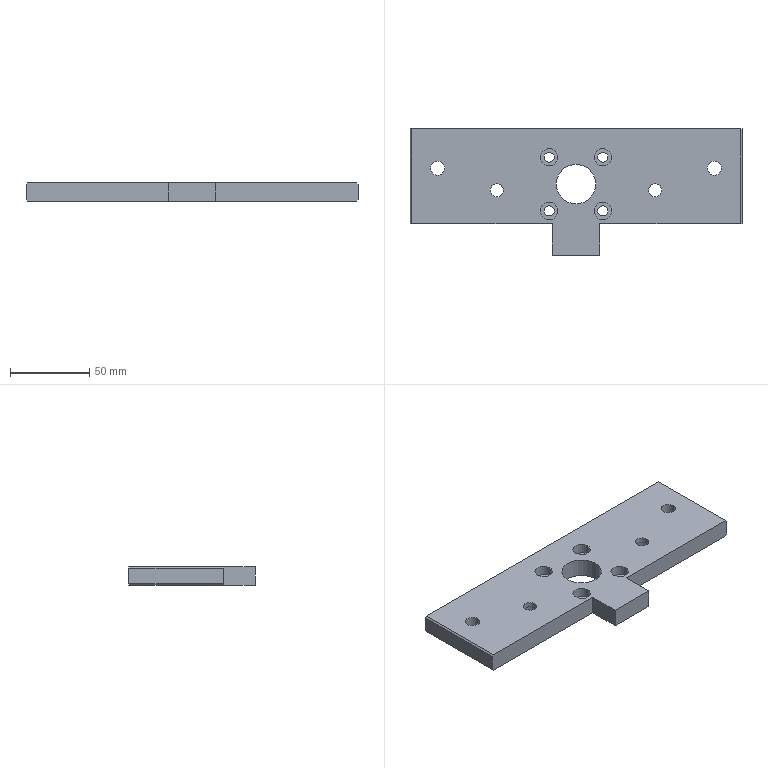Part | SolidWorks | features HoleWzd 3, Chamfer 1, Cut 1, Extrusion 1, ICE 1 | 1 solid | 50 faces | box 210 x 80 x 12 mm | volume 144293 mm3 | cylinder 30 | plane 20 | commonest cylinder face diameters 6.4 x8 11 x8 8.4 x4 9 x4 15 x4 25 x2
STEP:
#1=CARTESIAN_POINT('',(197.,35.,12.));
#2=VERTEX_POINT('',#1);
#3=CARTESIAN_POINT('',(188.,35.,12.));
#4=VERTEX_POINT('',#3);
#5=CARTESIAN_POINT('',(192.5,35.,12.));
#6=DIRECTION('',(0.,0.,-1.));
#7=DIRECTION('',(-1.,0.,0.));
#8=AXIS2_PLACEMENT_3D('',#5,#6,#7);
#9=CIRCLE('',#8,4.5);
#10=EDGE_CURVE('',#2,#4,#9,.T.);
#11=ORIENTED_EDGE('',*,*,#10,.F.);
#12=CARTESIAN_POINT('',(197.,35.,0.));
#13=VERTEX_POINT('',#12);
#14=CARTESIAN_POINT('',(197.,35.,0.));
#15=DIRECTION('',(0.,0.,-1.));
#16=VECTOR('',#15,1000.);
#17=LINE('',#14,#16);
#18=EDGE_CURVE('',#2,#13,#17,.T.);
#19=ORIENTED_EDGE('',*,*,#18,.T.);
#20=CARTESIAN_POINT('',(188.,35.,0.));
#21=VERTEX_POINT('',#20);
#22=CARTESIAN_POINT('',(192.5,35.,0.));
#23=DIRECTION('',(0.,0.,-1.));
#24=DIRECTION('',(-1.,0.,0.));
#25=AXIS2_PLACEMENT_3D('',#22,#23,#24);
#26=CIRCLE('',#25,4.5);
#27=EDGE_CURVE('',#13,#21,#26,.T.);
#28=ORIENTED_EDGE('',*,*,#27,.T.);
#29=CARTESIAN_POINT('',(188.,35.,0.));
#30=DIRECTION('',(0.,0.,-1.));
#31=VECTOR('',#30,1000.);
#32=LINE('',#29,#31);
#33=EDGE_CURVE('',#4,#21,#32,.T.);
#34=ORIENTED_EDGE('',*,*,#33,.F.);
#35=EDGE_LOOP('',(#11,#19,#28,#34));
#36=FACE_OUTER_BOUND('',#35,.T.);
#37=CARTESIAN_POINT('',(192.5,35.,0.));
#38=DIRECTION('',(0.,0.,-1.));
#39=DIRECTION('',(-1.,0.,0.));
#40=AXIS2_PLACEMENT_3D('',#37,#38,#39);
#41=CYLINDRICAL_SURFACE('',#40,4.5);
#42=ADVANCED_FACE('',(#36),#41,.F.);
#43=CARTESIAN_POINT('',(22.,35.,12.));
#44=VERTEX_POINT('',#43);
#45=CARTESIAN_POINT('',(13.,35.,12.));
#46=VERTEX_POINT('',#45);
#47=CARTESIAN_POINT('',(17.5,35.,12.));
#48=DIRECTION('',(0.,0.,-1.));
#49=DIRECTION('',(-1.,0.,0.));
#50=AXIS2_PLACEMENT_3D('',#47,#48,#49);
#51=CIRCLE('',#50,4.5);
#52=EDGE_CURVE('',#44,#46,#51,.T.);
#53=ORIENTED_EDGE('',*,*,#52,.F.);
#54=CARTESIAN_POINT('',(22.,35.,0.));
#55=VERTEX_POINT('',#54);
#56=CARTESIAN_POINT('',(22.,35.,0.));
#57=DIRECTION('',(0.,0.,-1.));
#58=VECTOR('',#57,1000.);
#59=LINE('',#56,#58);
#60=EDGE_CURVE('',#44,#55,#59,.T.);
#61=ORIENTED_EDGE('',*,*,#60,.T.);
#62=CARTESIAN_POINT('',(13.,35.,0.));
#63=VERTEX_POINT('',#62);
#64=CARTESIAN_POINT('',(17.5,35.,0.));
#65=DIRECTION('',(0.,0.,-1.));
#66=DIRECTION('',(-1.,0.,0.));
#67=AXIS2_PLACEMENT_3D('',#64,#65,#66);
#68=CIRCLE('',#67,4.5);
#69=EDGE_CURVE('',#55,#63,#68,.T.);
#70=ORIENTED_EDGE('',*,*,#69,.T.);
#71=CARTESIAN_POINT('',(13.,35.,0.));
#72=DIRECTION('',(0.,0.,-1.));
#73=VECTOR('',#72,1000.);
#74=LINE('',#71,#73);
#75=EDGE_CURVE('',#46,#63,#74,.T.);
#76=ORIENTED_EDGE('',*,*,#75,.F.);
#77=EDGE_LOOP('',(#53,#61,#70,#76));
#78=FACE_OUTER_BOUND('',#77,.T.);
#79=CARTESIAN_POINT('',(17.5,35.,0.));
#80=DIRECTION('',(0.,0.,-1.));
#81=DIRECTION('',(-1.,0.,0.));
#82=AXIS2_PLACEMENT_3D('',#79,#80,#81);
#83=CYLINDRICAL_SURFACE('',#82,4.5);
#84=ADVANCED_FACE('',(#78),#83,.F.);
#85=CARTESIAN_POINT('',(116.5,42.,5.6));
#86=VERTEX_POINT('',#85);
#87=CARTESIAN_POINT('',(127.5,42.,5.6));
#88=VERTEX_POINT('',#87);
#89=CARTESIAN_POINT('',(122.,42.,5.6));
#90=DIRECTION('',(0.,0.,1.));
#91=DIRECTION('',(1.,0.,0.));
#92=AXIS2_PLACEMENT_3D('',#89,#90,#91);
#93=CIRCLE('',#92,5.5);
#94=EDGE_CURVE('',#86,#88,#93,.T.);
#95=ORIENTED_EDGE('',*,*,#94,.F.);
#96=CARTESIAN_POINT('',(116.5,42.,12.));
#97=VERTEX_POINT('',#96);
#98=CARTESIAN_POINT('',(116.5,42.,12.));
#99=DIRECTION('',(0.,0.,1.));
#100=VECTOR('',#99,1000.);
#101=LINE('',#98,#100);
#102=EDGE_CURVE('',#86,#97,#101,.T.);
#103=ORIENTED_EDGE('',*,*,#102,.T.);
#104=CARTESIAN_POINT('',(127.5,42.,12.));
#105=VERTEX_POINT('',#104);
#106=CARTESIAN_POINT('',(122.,42.,12.));
#107=DIRECTION('',(0.,0.,1.));
#108=DIRECTION('',(1.,0.,0.));
#109=AXIS2_PLACEMENT_3D('',#106,#107,#108);
#110=CIRCLE('',#109,5.5);
#111=EDGE_CURVE('',#97,#105,#110,.T.);
#112=ORIENTED_EDGE('',*,*,#111,.T.);
#113=CARTESIAN_POINT('',(127.5,42.,12.));
#114=DIRECTION('',(0.,0.,1.));
#115=VECTOR('',#114,1000.);
#116=LINE('',#113,#115);
#117=EDGE_CURVE('',#88,#105,#116,.T.);
#118=ORIENTED_EDGE('',*,*,#117,.F.);
#119=EDGE_LOOP('',(#95,#103,#112,#118));
#120=FACE_OUTER_BOUND('',#119,.T.);
#121=CARTESIAN_POINT('',(122.,42.,12.));
#122=DIRECTION('',(0.,0.,1.));
#123=DIRECTION('',(1.,0.,0.));
#124=AXIS2_PLACEMENT_3D('',#121,#122,#123);
#125=CYLINDRICAL_SURFACE('',#124,5.5);
#126=ADVANCED_FACE('',(#120),#125,.F.);
#127=CARTESIAN_POINT('',(118.8,42.,0.));
#128=VERTEX_POINT('',#127);
#129=CARTESIAN_POINT('',(125.2,42.,0.));
#130=VERTEX_POINT('',#129);
#131=CARTESIAN_POINT('',(122.,42.,0.));
#132=DIRECTION('',(0.,0.,1.));
#133=DIRECTION('',(1.,0.,0.));
#134=AXIS2_PLACEMENT_3D('',#131,#132,#133);
#135=CIRCLE('',#134,3.2);
#136=EDGE_CURVE('',#128,#130,#135,.T.);
#137=ORIENTED_EDGE('',*,*,#136,.F.);
#138=CARTESIAN_POINT('',(118.8,42.,5.6));
#139=VERTEX_POINT('',#138);
#140=CARTESIAN_POINT('',(118.8,42.,12.));
#141=DIRECTION('',(0.,0.,1.));
#142=VECTOR('',#141,1000.);
#143=LINE('',#140,#142);
#144=EDGE_CURVE('',#128,#139,#143,.T.);
#145=ORIENTED_EDGE('',*,*,#144,.T.);
#146=CARTESIAN_POINT('',(125.2,42.,5.6));
#147=VERTEX_POINT('',#146);
#148=CARTESIAN_POINT('',(122.,42.,5.6));
#149=DIRECTION('',(0.,0.,1.));
#150=DIRECTION('',(1.,0.,0.));
#151=AXIS2_PLACEMENT_3D('',#148,#149,#150);
#152=CIRCLE('',#151,3.2);
#153=EDGE_CURVE('',#139,#147,#152,.T.);
#154=ORIENTED_EDGE('',*,*,#153,.T.);
#155=CARTESIAN_POINT('',(125.2,42.,12.));
#156=DIRECTION('',(0.,0.,1.));
#157=VECTOR('',#156,1000.);
#158=LINE('',#155,#157);
#159=EDGE_CURVE('',#130,#147,#158,.T.);
#160=ORIENTED_EDGE('',*,*,#159,.F.);
#161=EDGE_LOOP('',(#137,#145,#154,#160));
#162=FACE_OUTER_BOUND('',#161,.T.);
#163=CARTESIAN_POINT('',(122.,42.,12.));
#164=DIRECTION('',(0.,0.,1.));
#165=DIRECTION('',(1.,0.,0.));
#166=AXIS2_PLACEMENT_3D('',#163,#164,#165);
#167=CYLINDRICAL_SURFACE('',#166,3.2);
#168=ADVANCED_FACE('',(#162),#167,.F.);
#169=CARTESIAN_POINT('',(82.5,42.,5.6));
#170=VERTEX_POINT('',#169);
#171=CARTESIAN_POINT('',(93.5,42.,5.6));
#172=VERTEX_POINT('',#171);
#173=CARTESIAN_POINT('',(88.,42.,5.6));
#174=DIRECTION('',(0.,0.,1.));
#175=DIRECTION('',(1.,0.,0.));
#176=AXIS2_PLACEMENT_3D('',#173,#174,#175);
#177=CIRCLE('',#176,5.5);
#178=EDGE_CURVE('',#170,#172,#177,.T.);
#179=ORIENTED_EDGE('',*,*,#178,.F.);
#180=CARTESIAN_POINT('',(82.5,42.,12.));
#181=VERTEX_POINT('',#180);
#182=CARTESIAN_POINT('',(82.5,42.,12.));
#183=DIRECTION('',(0.,0.,1.));
#184=VECTOR('',#183,1000.);
#185=LINE('',#182,#184);
#186=EDGE_CURVE('',#170,#181,#185,.T.);
#187=ORIENTED_EDGE('',*,*,#186,.T.);
#188=CARTESIAN_POINT('',(93.5,42.,12.));
#189=VERTEX_POINT('',#188);
#190=CARTESIAN_POINT('',(88.,42.,12.));
#191=DIRECTION('',(0.,0.,1.));
#192=DIRECTION('',(1.,0.,0.));
#193=AXIS2_PLACEMENT_3D('',#190,#191,#192);
#194=CIRCLE('',#193,5.5);
#195=EDGE_CURVE('',#181,#189,#194,.T.);
#196=ORIENTED_EDGE('',*,*,#195,.T.);
#197=CARTESIAN_POINT('',(93.5,42.,12.));
#198=DIRECTION('',(0.,0.,1.));
#199=VECTOR('',#198,1000.);
#200=LINE('',#197,#199);
#201=EDGE_CURVE('',#172,#189,#200,.T.);
#202=ORIENTED_EDGE('',*,*,#201,.F.);
#203=EDGE_LOOP('',(#179,#187,#196,#202));
#204=FACE_OUTER_BOUND('',#203,.T.);
#205=CARTESIAN_POINT('',(88.,42.,12.));
#206=DIRECTION('',(0.,0.,1.));
#207=DIRECTION('',(1.,0.,0.));
#208=AXIS2_PLACEMENT_3D('',#205,#206,#207);
#209=CYLINDRICAL_SURFACE('',#208,5.5);
#210=ADVANCED_FACE('',(#204),#209,.F.);
#211=CARTESIAN_POINT('',(84.8,42.,0.));
#212=VERTEX_POINT('',#211);
#213=CARTESIAN_POINT('',(91.2,42.,0.));
#214=VERTEX_POINT('',#213);
#215=CARTESIAN_POINT('',(88.,42.,0.));
#216=DIRECTION('',(0.,0.,1.));
#217=DIRECTION('',(1.,0.,0.));
#218=AXIS2_PLACEMENT_3D('',#215,#216,#217);
#219=CIRCLE('',#218,3.2);
#220=EDGE_CURVE('',#212,#214,#219,.T.);
#221=ORIENTED_EDGE('',*,*,#220,.F.);
#222=CARTESIAN_POINT('',(84.8,42.,5.6));
#223=VERTEX_POINT('',#222);
#224=CARTESIAN_POINT('',(84.8,42.,12.));
#225=DIRECTION('',(0.,0.,1.));
#226=VECTOR('',#225,1000.);
#227=LINE('',#224,#226);
#228=EDGE_CURVE('',#212,#223,#227,.T.);
#229=ORIENTED_EDGE('',*,*,#228,.T.);
#230=CARTESIAN_POINT('',(91.2,42.,5.6));
#231=VERTEX_POINT('',#230);
#232=CARTESIAN_POINT('',(88.,42.,5.6));
#233=DIRECTION('',(0.,0.,1.));
#234=DIRECTION('',(1.,0.,0.));
#235=AXIS2_PLACEMENT_3D('',#232,#233,#234);
#236=CIRCLE('',#235,3.2);
#237=EDGE_CURVE('',#223,#231,#236,.T.);
#238=ORIENTED_EDGE('',*,*,#237,.T.);
#239=CARTESIAN_POINT('',(91.2,42.,12.));
#240=DIRECTION('',(0.,0.,1.));
#241=VECTOR('',#240,1000.);
#242=LINE('',#239,#241);
#243=EDGE_CURVE('',#214,#231,#242,.T.);
#244=ORIENTED_EDGE('',*,*,#243,.F.);
#245=EDGE_LOOP('',(#221,#229,#238,#244));
#246=FACE_OUTER_BOUND('',#245,.T.);
#247=CARTESIAN_POINT('',(88.,42.,12.));
#248=DIRECTION('',(0.,0.,1.));
#249=DIRECTION('',(1.,0.,0.));
#250=AXIS2_PLACEMENT_3D('',#247,#248,#249);
#251=CYLINDRICAL_SURFACE('',#250,3.2);
#252=ADVANCED_FACE('',(#246),#251,.F.);
#253=CARTESIAN_POINT('',(116.5,8.,5.6));
#254=VERTEX_POINT('',#253);
#255=CARTESIAN_POINT('',(127.5,8.,5.6));
#256=VERTEX_POINT('',#255);
#257=CARTESIAN_POINT('',(122.,8.,5.6));
#258=DIRECTION('',(0.,0.,1.));
#259=DIRECTION('',(1.,0.,0.));
#260=AXIS2_PLACEMENT_3D('',#257,#258,#259);
#261=CIRCLE('',#260,5.5);
#262=EDGE_CURVE('',#254,#256,#261,.T.);
#263=ORIENTED_EDGE('',*,*,#262,.F.);
#264=CARTESIAN_POINT('',(116.5,8.,12.));
#265=VERTEX_POINT('',#264);
#266=CARTESIAN_POINT('',(116.5,8.,12.));
#267=DIRECTION('',(0.,0.,1.));
#268=VECTOR('',#267,1000.);
#269=LINE('',#266,#268);
#270=EDGE_CURVE('',#254,#265,#269,.T.);
#271=ORIENTED_EDGE('',*,*,#270,.T.);
#272=CARTESIAN_POINT('',(127.5,8.,12.));
#273=VERTEX_POINT('',#272);
#274=CARTESIAN_POINT('',(122.,8.,12.));
#275=DIRECTION('',(0.,0.,1.));
#276=DIRECTION('',(1.,0.,0.));
#277=AXIS2_PLACEMENT_3D('',#274,#275,#276);
#278=CIRCLE('',#277,5.5);
#279=EDGE_CURVE('',#265,#273,#278,.T.);
#280=ORIENTED_EDGE('',*,*,#279,.T.);
#281=CARTESIAN_POINT('',(127.5,8.,12.));
#282=DIRECTION('',(0.,0.,1.));
#283=VECTOR('',#282,1000.);
#284=LINE('',#281,#283);
#285=EDGE_CURVE('',#256,#273,#284,.T.);
#286=ORIENTED_EDGE('',*,*,#285,.F.);
#287=EDGE_LOOP('',(#263,#271,#280,#286));
#288=FACE_OUTER_BOUND('',#287,.T.);
#289=CARTESIAN_POINT('',(122.,8.,12.));
#290=DIRECTION('',(0.,0.,1.));
#291=DIRECTION('',(1.,0.,0.));
#292=AXIS2_PLACEMENT_3D('',#289,#290,#291);
#293=CYLINDRICAL_SURFACE('',#292,5.5);
#294=ADVANCED_FACE('',(#288),#293,.F.);
#295=CARTESIAN_POINT('',(118.8,8.,0.));
#296=VERTEX_POINT('',#295);
#297=CARTESIAN_POINT('',(125.2,8.,0.));
#298=VERTEX_POINT('',#297);
#299=CARTESIAN_POINT('',(122.,8.,0.));
#300=DIRECTION('',(0.,0.,1.));
#301=DIRECTION('',(1.,0.,0.));
#302=AXIS2_PLACEMENT_3D('',#299,#300,#301);
#303=CIRCLE('',#302,3.2);
#304=EDGE_CURVE('',#296,#298,#303,.T.);
#305=ORIENTED_EDGE('',*,*,#304,.F.);
#306=CARTESIAN_POINT('',(118.8,8.,5.6));
#307=VERTEX_POINT('',#306);
#308=CARTESIAN_POINT('',(118.8,8.,12.));
#309=DIRECTION('',(0.,0.,1.));
#310=VECTOR('',#309,1000.);
#311=LINE('',#308,#310);
#312=EDGE_CURVE('',#296,#307,#311,.T.);
#313=ORIENTED_EDGE('',*,*,#312,.T.);
#314=CARTESIAN_POINT('',(125.2,8.,5.6));
#315=VERTEX_POINT('',#314);
#316=CARTESIAN_POINT('',(122.,8.,5.6));
#317=DIRECTION('',(0.,0.,1.));
#318=DIRECTION('',(1.,0.,0.));
#319=AXIS2_PLACEMENT_3D('',#316,#317,#318);
#320=CIRCLE('',#319,3.2);
#321=EDGE_CURVE('',#307,#315,#320,.T.);
#322=ORIENTED_EDGE('',*,*,#321,.T.);
#323=CARTESIAN_POINT('',(125.2,8.,12.));
#324=DIRECTION('',(0.,0.,1.));
#325=VECTOR('',#324,1000.);
#326=LINE('',#323,#325);
#327=EDGE_CURVE('',#298,#315,#326,.T.);
#328=ORIENTED_EDGE('',*,*,#327,.F.);
#329=EDGE_LOOP('',(#305,#313,#322,#328));
#330=FACE_OUTER_BOUND('',#329,.T.);
#331=CARTESIAN_POINT('',(122.,8.,12.));
#332=DIRECTION('',(0.,0.,1.));
#333=DIRECTION('',(1.,0.,0.));
#334=AXIS2_PLACEMENT_3D('',#331,#332,#333);
#335=CYLINDRICAL_SURFACE('',#334,3.2);
#336=ADVANCED_FACE('',(#330),#335,.F.);
#337=CARTESIAN_POINT('',(82.5,8.,5.6));
#338=VERTEX_POINT('',#337);
#339=CARTESIAN_POINT('',(93.5,8.,5.6));
#340=VERTEX_POINT('',#339);
#341=CARTESIAN_POINT('',(88.,8.,5.6));
#342=DIRECTION('',(0.,0.,1.));
#343=DIRECTION('',(1.,0.,0.));
#344=AXIS2_PLACEMENT_3D('',#341,#342,#343);
#345=CIRCLE('',#344,5.5);
#346=EDGE_CURVE('',#338,#340,#345,.T.);
#347=ORIENTED_EDGE('',*,*,#346,.F.);
#348=CARTESIAN_POINT('',(82.5,8.,12.));
#349=VERTEX_POINT('',#348);
#350=CARTESIAN_POINT('',(82.5,8.,12.));
#351=DIRECTION('',(0.,0.,1.));
#352=VECTOR('',#351,1000.);
#353=LINE('',#350,#352);
#354=EDGE_CURVE('',#338,#349,#353,.T.);
#355=ORIENTED_EDGE('',*,*,#354,.T.);
#356=CARTESIAN_POINT('',(93.5,8.,12.));
#357=VERTEX_POINT('',#356);
#358=CARTESIAN_POINT('',(88.,8.,12.));
#359=DIRECTION('',(0.,0.,1.));
#360=DIRECTION('',(1.,0.,0.));
#361=AXIS2_PLACEMENT_3D('',#358,#359,#360);
#362=CIRCLE('',#361,5.5);
#363=EDGE_CURVE('',#349,#357,#362,.T.);
#364=ORIENTED_EDGE('',*,*,#363,.T.);
#365=CARTESIAN_POINT('',(93.5,8.,12.));
#366=DIRECTION('',(0.,0.,1.));
#367=VECTOR('',#366,1000.);
#368=LINE('',#365,#367);
#369=EDGE_CURVE('',#340,#357,#368,.T.);
#370=ORIENTED_EDGE('',*,*,#369,.F.);
#371=EDGE_LOOP('',(#347,#355,#364,#370));
#372=FACE_OUTER_BOUND('',#371,.T.);
#373=CARTESIAN_POINT('',(88.,8.,12.));
#374=DIRECTION('',(0.,0.,1.));
#375=DIRECTION('',(1.,0.,0.));
#376=AXIS2_PLACEMENT_3D('',#373,#374,#375);
#377=CYLINDRICAL_SURFACE('',#376,5.5);
#378=ADVANCED_FACE('',(#372),#377,.F.);
#379=CARTESIAN_POINT('',(84.8,8.,0.));
#380=VERTEX_POINT('',#379);
#381=CARTESIAN_POINT('',(91.2,8.,0.));
#382=VERTEX_POINT('',#381);
#383=CARTESIAN_POINT('',(88.,8.,0.));
#384=DIRECTION('',(0.,0.,1.));
#385=DIRECTION('',(1.,0.,0.));
#386=AXIS2_PLACEMENT_3D('',#383,#384,#385);
#387=CIRCLE('',#386,3.2);
#388=EDGE_CURVE('',#380,#382,#387,.T.);
#389=ORIENTED_EDGE('',*,*,#388,.F.);
#390=CARTESIAN_POINT('',(84.8,8.,5.6));
#391=VERTEX_POINT('',#390);
#392=CARTESIAN_POINT('',(84.8,8.,12.));
#393=DIRECTION('',(0.,0.,1.));
#394=VECTOR('',#393,1000.);
#395=LINE('',#392,#394);
#396=EDGE_CURVE('',#380,#391,#395,.T.);
#397=ORIENTED_EDGE('',*,*,#396,.T.);
#398=CARTESIAN_POINT('',(91.2,8.,5.6));
#399=VERTEX_POINT('',#398);
#400=CARTESIAN_POINT('',(88.,8.,5.6));
#401=DIRECTION('',(0.,0.,1.));
#402=DIRECTION('',(1.,0.,0.));
#403=AXIS2_PLACEMENT_3D('',#400,#401,#402);
#404=CIRCLE('',#403,3.2);
#405=EDGE_CURVE('',#391,#399,#404,.T.);
#406=ORIENTED_EDGE('',*,*,#405,.T.);
#407=CARTESIAN_POINT('',(91.2,8.,12.));
#408=DIRECTION('',(0.,0.,1.));
#409=VECTOR('',#408,1000.);
#410=LINE('',#407,#409);
#411=EDGE_CURVE('',#382,#399,#410,.T.);
#412=ORIENTED_EDGE('',*,*,#411,.F.);
#413=EDGE_LOOP('',(#389,#397,#406,#412));
#414=FACE_OUTER_BOUND('',#413,.T.);
#415=CARTESIAN_POINT('',(88.,8.,12.));
#416=DIRECTION('',(0.,0.,1.));
#417=DIRECTION('',(1.,0.,0.));
#418=AXIS2_PLACEMENT_3D('',#415,#416,#417);
#419=CYLINDRICAL_SURFACE('',#418,3.2);
#420=ADVANCED_FACE('',(#414),#419,.F.);
#421=CARTESIAN_POINT('',(62.5,21.,8.6));
#422=VERTEX_POINT('',#421);
#423=CARTESIAN_POINT('',(47.5,21.,8.6));
#424=VERTEX_POINT('',#423);
#425=CARTESIAN_POINT('',(55.,21.,8.6));
#426=DIRECTION('',(0.,0.,-1.));
#427=DIRECTION('',(-1.,0.,0.));
#428=AXIS2_PLACEMENT_3D('',#425,#426,#427);
#429=CIRCLE('',#428,7.5);
#430=EDGE_CURVE('',#422,#424,#429,.T.);
#431=ORIENTED_EDGE('',*,*,#430,.F.);
#432=CARTESIAN_POINT('',(62.5,21.,0.));
#433=VERTEX_POINT('',#432);
#434=CARTESIAN_POINT('',(62.5,21.,0.));
#435=DIRECTION('',(0.,0.,-1.));
#436=VECTOR('',#435,1000.);
#437=LINE('',#434,#436);
#438=EDGE_CURVE('',#422,#433,#437,.T.);
#439=ORIENTED_EDGE('',*,*,#438,.T.);
#440=CARTESIAN_POINT('',(47.5,21.,0.));
#441=VERTEX_POINT('',#440);
#442=CARTESIAN_POINT('',(55.,21.,0.));
#443=DIRECTION('',(0.,0.,-1.));
#444=DIRECTION('',(-1.,0.,0.));
#445=AXIS2_PLACEMENT_3D('',#442,#443,#444);
#446=CIRCLE('',#445,7.5);
#447=EDGE_CURVE('',#433,#441,#446,.T.);
#448=ORIENTED_EDGE('',*,*,#447,.T.);
#449=CARTESIAN_POINT('',(47.5,21.,0.));
#450=DIRECTION('',(0.,0.,-1.));
#451=VECTOR('',#450,1000.);
#452=LINE('',#449,#451);
#453=EDGE_CURVE('',#424,#441,#452,.T.);
#454=ORIENTED_EDGE('',*,*,#453,.F.);
#455=EDGE_LOOP('',(#431,#439,#448,#454));
#456=FACE_OUTER_BOUND('',#455,.T.);
#457=CARTESIAN_POINT('',(55.,21.,0.));
#458=DIRECTION('',(0.,0.,-1.));
#459=DIRECTION('',(-1.,0.,0.));
#460=AXIS2_PLACEMENT_3D('',#457,#458,#459);
#461=CYLINDRICAL_SURFACE('',#460,7.5);
#462=ADVANCED_FACE('',(#456),#461,.F.);
#463=CARTESIAN_POINT('',(59.2,21.,12.));
#464=VERTEX_POINT('',#463);
#465=CARTESIAN_POINT('',(50.8,21.,12.));
#466=VERTEX_POINT('',#465);
#467=CARTESIAN_POINT('',(55.,21.,12.));
#468=DIRECTION('',(0.,0.,-1.));
#469=DIRECTION('',(-1.,0.,0.));
#470=AXIS2_PLACEMENT_3D('',#467,#468,#469);
#471=CIRCLE('',#470,4.2);
#472=EDGE_CURVE('',#464,#466,#471,.T.);
#473=ORIENTED_EDGE('',*,*,#472,.F.);
#474=CARTESIAN_POINT('',(59.2,21.,8.6));
#475=VERTEX_POINT('',#474);
#476=CARTESIAN_POINT('',(59.2,21.,0.));
#477=DIRECTION('',(0.,0.,-1.));
#478=VECTOR('',#477,1000.);
#479=LINE('',#476,#478);
#480=EDGE_CURVE('',#464,#475,#479,.T.);
#481=ORIENTED_EDGE('',*,*,#480,.T.);
#482=CARTESIAN_POINT('',(50.8,21.,8.6));
#483=VERTEX_POINT('',#482);
#484=CARTESIAN_POINT('',(55.,21.,8.6));
#485=DIRECTION('',(0.,0.,-1.));
#486=DIRECTION('',(-1.,0.,0.));
#487=AXIS2_PLACEMENT_3D('',#484,#485,#486);
#488=CIRCLE('',#487,4.2);
#489=EDGE_CURVE('',#475,#483,#488,.T.);
#490=ORIENTED_EDGE('',*,*,#489,.T.);
#491=CARTESIAN_POINT('',(50.8,21.,0.));
#492=DIRECTION('',(0.,0.,-1.));
#493=VECTOR('',#492,1000.);
#494=LINE('',#491,#493);
#495=EDGE_CURVE('',#466,#483,#494,.T.);
#496=ORIENTED_EDGE('',*,*,#495,.F.);
#497=EDGE_LOOP('',(#473,#481,#490,#496));
#498=FACE_OUTER_BOUND('',#497,.T.);
#499=CARTESIAN_POINT('',(55.,21.,0.));
#500=DIRECTION('',(0.,0.,-1.));
#501=DIRECTION('',(-1.,0.,0.));
#502=AXIS2_PLACEMENT_3D('',#499,#500,#501);
#503=CYLINDRICAL_SURFACE('',#502,4.2);
#504=ADVANCED_FACE('',(#498),#503,.F.);
#505=CARTESIAN_POINT('',(162.5,21.,8.6));
#506=VERTEX_POINT('',#505);
#507=CARTESIAN_POINT('',(147.5,21.,8.6));
#508=VERTEX_POINT('',#507);
#509=CARTESIAN_POINT('',(155.,21.,8.6));
#510=DIRECTION('',(0.,0.,-1.));
#511=DIRECTION('',(-1.,0.,0.));
#512=AXIS2_PLACEMENT_3D('',#509,#510,#511);
#513=CIRCLE('',#512,7.5);
#514=EDGE_CURVE('',#506,#508,#513,.T.);
#515=ORIENTED_EDGE('',*,*,#514,.F.);
#516=CARTESIAN_POINT('',(162.5,21.,0.));
#517=VERTEX_POINT('',#516);
#518=CARTESIAN_POINT('',(162.5,21.,0.));
#519=DIRECTION('',(0.,0.,-1.));
#520=VECTOR('',#519,1000.);
#521=LINE('',#518,#520);
#522=EDGE_CURVE('',#506,#517,#521,.T.);
#523=ORIENTED_EDGE('',*,*,#522,.T.);
#524=CARTESIAN_POINT('',(147.5,21.,0.));
#525=VERTEX_POINT('',#524);
#526=CARTESIAN_POINT('',(155.,21.,0.));
#527=DIRECTION('',(0.,0.,-1.));
#528=DIRECTION('',(-1.,0.,0.));
#529=AXIS2_PLACEMENT_3D('',#526,#527,#528);
#530=CIRCLE('',#529,7.5);
#531=EDGE_CURVE('',#517,#525,#530,.T.);
#532=ORIENTED_EDGE('',*,*,#531,.T.);
#533=CARTESIAN_POINT('',(147.5,21.,0.));
#534=DIRECTION('',(0.,0.,-1.));
#535=VECTOR('',#534,1000.);
#536=LINE('',#533,#535);
#537=EDGE_CURVE('',#508,#525,#536,.T.);
#538=ORIENTED_EDGE('',*,*,#537,.F.);
#539=EDGE_LOOP('',(#515,#523,#532,#538));
#540=FACE_OUTER_BOUND('',#539,.T.);
#541=CARTESIAN_POINT('',(155.,21.,0.));
#542=DIRECTION('',(0.,0.,-1.));
#543=DIRECTION('',(-1.,0.,0.));
#544=AXIS2_PLACEMENT_3D('',#541,#542,#543);
#545=CYLINDRICAL_SURFACE('',#544,7.5);
#546=ADVANCED_FACE('',(#540),#545,.F.);
#547=CARTESIAN_POINT('',(159.2,21.,12.));
#548=VERTEX_POINT('',#547);
#549=CARTESIAN_POINT('',(150.8,21.,12.));
#550=VERTEX_POINT('',#549);
#551=CARTESIAN_POINT('',(155.,21.,12.));
#552=DIRECTION('',(0.,0.,-1.));
#553=DIRECTION('',(-1.,0.,0.));
#554=AXIS2_PLACEMENT_3D('',#551,#552,#553);
#555=CIRCLE('',#554,4.2);
#556=EDGE_CURVE('',#548,#550,#555,.T.);
#557=ORIENTED_EDGE('',*,*,#556,.F.);
#558=CARTESIAN_POINT('',(159.2,21.,8.6));
#559=VERTEX_POINT('',#558);
#560=CARTESIAN_POINT('',(159.2,21.,0.));
#561=DIRECTION('',(0.,0.,-1.));
#562=VECTOR('',#561,1000.);
#563=LINE('',#560,#562);
#564=EDGE_CURVE('',#548,#559,#563,.T.);
#565=ORIENTED_EDGE('',*,*,#564,.T.);
#566=CARTESIAN_POINT('',(150.8,21.,8.6));
#567=VERTEX_POINT('',#566);
#568=CARTESIAN_POINT('',(155.,21.,8.6));
#569=DIRECTION('',(0.,0.,-1.));
#570=DIRECTION('',(-1.,0.,0.));
#571=AXIS2_PLACEMENT_3D('',#568,#569,#570);
#572=CIRCLE('',#571,4.2);
#573=EDGE_CURVE('',#559,#567,#572,.T.);
#574=ORIENTED_EDGE('',*,*,#573,.T.);
#575=CARTESIAN_POINT('',(150.8,21.,0.));
#576=DIRECTION('',(0.,0.,-1.));
#577=VECTOR('',#576,1000.);
#578=LINE('',#575,#577);
#579=EDGE_CURVE('',#550,#567,#578,.T.);
#580=ORIENTED_EDGE('',*,*,#579,.F.);
#581=EDGE_LOOP('',(#557,#565,#574,#580));
#582=FACE_OUTER_BOUND('',#581,.T.);
#583=CARTESIAN_POINT('',(155.,21.,0.));
#584=DIRECTION('',(0.,0.,-1.));
#585=DIRECTION('',(-1.,0.,0.));
#586=AXIS2_PLACEMENT_3D('',#583,#584,#585);
#587=CYLINDRICAL_SURFACE('',#586,4.2);
#588=ADVANCED_FACE('',(#582),#587,.F.);
#589=CARTESIAN_POINT('',(92.5,25.,0.));
#590=VERTEX_POINT('',#589);
#591=CARTESIAN_POINT('',(117.5,25.,0.));
#592=VERTEX_POINT('',#591);
#593=CARTESIAN_POINT('',(105.,25.,0.));
#594=DIRECTION('',(0.,0.,1.));
#595=DIRECTION('',(1.,0.,0.));
#596=AXIS2_PLACEMENT_3D('',#593,#594,#595);
#597=CIRCLE('',#596,12.5);
#598=EDGE_CURVE('',#590,#592,#597,.T.);
#599=ORIENTED_EDGE('',*,*,#598,.F.);
#600=CARTESIAN_POINT('',(92.5,25.,12.));
#601=VERTEX_POINT('',#600);
#602=CARTESIAN_POINT('',(92.5,25.,0.));
#603=DIRECTION('',(0.,0.,1.));
#604=VECTOR('',#603,1000.);
#605=LINE('',#602,#604);
#606=EDGE_CURVE('',#590,#601,#605,.T.);
#607=ORIENTED_EDGE('',*,*,#606,.T.);
#608=CARTESIAN_POINT('',(117.5,25.,12.));
#609=VERTEX_POINT('',#608);
#610=CARTESIAN_POINT('',(105.,25.,12.));
#611=DIRECTION('',(0.,0.,1.));
#612=DIRECTION('',(1.,0.,0.));
#613=AXIS2_PLACEMENT_3D('',#610,#611,#612);
#614=CIRCLE('',#613,12.5);
#615=EDGE_CURVE('',#601,#609,#614,.T.);
#616=ORIENTED_EDGE('',*,*,#615,.T.);
#617=CARTESIAN_POINT('',(117.5,25.,0.));
#618=DIRECTION('',(0.,0.,1.));
#619=VECTOR('',#618,1000.);
#620=LINE('',#617,#619);
#621=EDGE_CURVE('',#592,#609,#620,.T.);
#622=ORIENTED_EDGE('',*,*,#621,.F.);
#623=EDGE_LOOP('',(#599,#607,#616,#622));
#624=FACE_OUTER_BOUND('',#623,.T.);
#625=CARTESIAN_POINT('',(105.,25.,0.));
#626=DIRECTION('',(0.,0.,1.));
#627=DIRECTION('',(1.,0.,0.));
#628=AXIS2_PLACEMENT_3D('',#625,#626,#627);
#629=CYLINDRICAL_SURFACE('',#628,12.5);
#630=ADVANCED_FACE('',(#624),#629,.F.);
#631=CARTESIAN_POINT('',(90.,0.,12.));
#632=VERTEX_POINT('',#631);
#633=CARTESIAN_POINT('',(90.,0.,0.));
#634=VERTEX_POINT('',#633);
#635=CARTESIAN_POINT('',(90.,0.,48.056));
#636=DIRECTION('',(0.,0.,-1.));
#637=VECTOR('',#636,1000.);
#638=LINE('',#635,#637);
#639=EDGE_CURVE('',#632,#634,#638,.T.);
#640=ORIENTED_EDGE('',*,*,#639,.F.);
#641=CARTESIAN_POINT('',(1.,0.,12.));
#642=VERTEX_POINT('',#641);
#643=CARTESIAN_POINT('',(0.,0.,12.));
#644=DIRECTION('',(1.,0.,0.));
#645=VECTOR('',#644,1000.);
#646=LINE('',#643,#645);
#647=EDGE_CURVE('',#642,#632,#646,.T.);
#648=ORIENTED_EDGE('',*,*,#647,.F.);
#649=CARTESIAN_POINT('',(0.,0.,11.));
#650=VERTEX_POINT('',#649);
#651=CARTESIAN_POINT('',(1.,0.,12.));
#652=DIRECTION('',(-0.7071,0.,-0.7071));
#653=VECTOR('',#652,1000.);
#654=LINE('',#651,#653);
#655=EDGE_CURVE('',#642,#650,#654,.T.);
#656=ORIENTED_EDGE('',*,*,#655,.T.);
#657=CARTESIAN_POINT('',(0.,0.,1.));
#658=VERTEX_POINT('',#657);
#659=CARTESIAN_POINT('',(0.,0.,12.));
#660=DIRECTION('',(0.,0.,-1.));
#661=VECTOR('',#660,1000.);
#662=LINE('',#659,#661);
#663=EDGE_CURVE('',#650,#658,#662,.T.);
#664=ORIENTED_EDGE('',*,*,#663,.T.);
#665=CARTESIAN_POINT('',(1.,0.,0.));
#666=VERTEX_POINT('',#665);
#667=CARTESIAN_POINT('',(0.,0.,1.));
#668=DIRECTION('',(0.7071,0.,-0.7071));
#669=VECTOR('',#668,1000.);
#670=LINE('',#667,#669);
#671=EDGE_CURVE('',#658,#666,#670,.T.);
#672=ORIENTED_EDGE('',*,*,#671,.T.);
#673=CARTESIAN_POINT('',(0.,0.,0.));
#674=DIRECTION('',(1.,0.,0.));
#675=VECTOR('',#674,1000.);
#676=LINE('',#673,#675);
#677=EDGE_CURVE('',#666,#634,#676,.T.);
#678=ORIENTED_EDGE('',*,*,#677,.T.);
#679=EDGE_LOOP('',(#640,#648,#656,#664,#672,#678));
#680=FACE_OUTER_BOUND('',#679,.T.);
#681=CARTESIAN_POINT('',(0.,0.,12.));
#682=DIRECTION('',(0.,1.,0.));
#683=DIRECTION('',(0.,0.,1.));
#684=AXIS2_PLACEMENT_3D('',#681,#682,#683);
#685=PLANE('',#684);
#686=ADVANCED_FACE('',(#680),#685,.F.);
#687=CARTESIAN_POINT('',(0.,60.,11.));
#688=VERTEX_POINT('',#687);
#689=CARTESIAN_POINT('',(0.,60.,1.));
#690=VERTEX_POINT('',#689);
#691=CARTESIAN_POINT('',(0.,60.,12.));
#692=DIRECTION('',(0.,0.,-1.));
#693=VECTOR('',#692,1000.);
#694=LINE('',#691,#693);
#695=EDGE_CURVE('',#688,#690,#694,.T.);
#696=ORIENTED_EDGE('',*,*,#695,.T.);
#697=CARTESIAN_POINT('',(0.,0.,1.));
#698=DIRECTION('',(0.,-1.,0.));
#699=VECTOR('',#698,1000.);
#700=LINE('',#697,#699);
#701=EDGE_CURVE('',#690,#658,#700,.T.);
#702=ORIENTED_EDGE('',*,*,#701,.T.);
#703=ORIENTED_EDGE('',*,*,#663,.F.);
#704=CARTESIAN_POINT('',(0.,0.,11.));
#705=DIRECTION('',(0.,1.,0.));
#706=VECTOR('',#705,1000.);
#707=LINE('',#704,#706);
#708=EDGE_CURVE('',#650,#688,#707,.T.);
#709=ORIENTED_EDGE('',*,*,#708,.T.);
#710=EDGE_LOOP('',(#696,#702,#703,#709));
#711=FACE_OUTER_BOUND('',#710,.T.);
#712=CARTESIAN_POINT('',(0.,0.,12.));
#713=DIRECTION('',(1.,0.,0.));
#714=DIRECTION('',(0.,0.,-1.));
#715=AXIS2_PLACEMENT_3D('',#712,#713,#714);
#716=PLANE('',#715);
#717=ADVANCED_FACE('',(#711),#716,.F.);
#718=CARTESIAN_POINT('',(120.,0.,12.));
#719=VERTEX_POINT('',#718);
#720=CARTESIAN_POINT('',(209.,0.,12.));
#721=VERTEX_POINT('',#720);
#722=CARTESIAN_POINT('',(0.,0.,12.));
#723=DIRECTION('',(1.,0.,0.));
#724=VECTOR('',#723,1000.);
#725=LINE('',#722,#724);
#726=EDGE_CURVE('',#719,#721,#725,.T.);
#727=ORIENTED_EDGE('',*,*,#726,.F.);
#728=CARTESIAN_POINT('',(120.,0.,0.));
#729=VERTEX_POINT('',#728);
#730=CARTESIAN_POINT('',(120.,0.,48.056));
#731=DIRECTION('',(0.,0.,-1.));
#732=VECTOR('',#731,1000.);
#733=LINE('',#730,#732);
#734=EDGE_CURVE('',#719,#729,#733,.T.);
#735=ORIENTED_EDGE('',*,*,#734,.T.);
#736=CARTESIAN_POINT('',(209.,0.,0.));
#737=VERTEX_POINT('',#736);
#738=CARTESIAN_POINT('',(0.,0.,0.));
#739=DIRECTION('',(1.,0.,0.));
#740=VECTOR('',#739,1000.);
#741=LINE('',#738,#740);
#742=EDGE_CURVE('',#729,#737,#741,.T.);
#743=ORIENTED_EDGE('',*,*,#742,.T.);
#744=CARTESIAN_POINT('',(210.,0.,1.));
#745=VERTEX_POINT('',#744);
#746=CARTESIAN_POINT('',(210.,0.,1.));
#747=DIRECTION('',(0.7071,0.,0.7071));
#748=VECTOR('',#747,1000.);
#749=LINE('',#746,#748);
#750=EDGE_CURVE('',#737,#745,#749,.T.);
#751=ORIENTED_EDGE('',*,*,#750,.T.);
#752=CARTESIAN_POINT('',(210.,0.,11.));
#753=VERTEX_POINT('',#752);
#754=CARTESIAN_POINT('',(210.,0.,12.));
#755=DIRECTION('',(0.,0.,-1.));
#756=VECTOR('',#755,1000.);
#757=LINE('',#754,#756);
#758=EDGE_CURVE('',#753,#745,#757,.T.);
#759=ORIENTED_EDGE('',*,*,#758,.F.);
#760=CARTESIAN_POINT('',(209.,0.,12.));
#761=DIRECTION('',(-0.7071,0.,0.7071));
#762=VECTOR('',#761,1000.);
#763=LINE('',#760,#762);
#764=EDGE_CURVE('',#753,#721,#763,.T.);
#765=ORIENTED_EDGE('',*,*,#764,.T.);
#766=EDGE_LOOP('',(#727,#735,#743,#751,#759,#765));
#767=FACE_OUTER_BOUND('',#766,.T.);
#768=CARTESIAN_POINT('',(0.,0.,12.));
#769=DIRECTION('',(0.,1.,0.));
#770=DIRECTION('',(0.,0.,1.));
#771=AXIS2_PLACEMENT_3D('',#768,#769,#770);
#772=PLANE('',#771);
#773=ADVANCED_FACE('',(#767),#772,.F.);
#774=ORIENTED_EDGE('',*,*,#758,.T.);
#775=CARTESIAN_POINT('',(210.,60.,1.));
#776=VERTEX_POINT('',#775);
#777=CARTESIAN_POINT('',(210.,60.,1.));
#778=DIRECTION('',(0.,1.,0.));
#779=VECTOR('',#778,1000.);
#780=LINE('',#777,#779);
#781=EDGE_CURVE('',#745,#776,#780,.T.);
#782=ORIENTED_EDGE('',*,*,#781,.T.);
#783=CARTESIAN_POINT('',(210.,60.,11.));
#784=VERTEX_POINT('',#783);
#785=CARTESIAN_POINT('',(210.,60.,12.));
#786=DIRECTION('',(0.,0.,-1.));
#787=VECTOR('',#786,1000.);
#788=LINE('',#785,#787);
#789=EDGE_CURVE('',#784,#776,#788,.T.);
#790=ORIENTED_EDGE('',*,*,#789,.F.);
#791=CARTESIAN_POINT('',(210.,0.,11.));
#792=DIRECTION('',(0.,-1.,0.));
#793=VECTOR('',#792,1000.);
#794=LINE('',#791,#793);
#795=EDGE_CURVE('',#784,#753,#794,.T.);
#796=ORIENTED_EDGE('',*,*,#795,.T.);
#797=EDGE_LOOP('',(#774,#782,#790,#796));
#798=FACE_OUTER_BOUND('',#797,.T.);
#799=CARTESIAN_POINT('',(210.,0.,12.));
#800=DIRECTION('',(-1.,0.,0.));
#801=DIRECTION('',(0.,0.,1.));
#802=AXIS2_PLACEMENT_3D('',#799,#800,#801);
#803=PLANE('',#802);
#804=ADVANCED_FACE('',(#798),#803,.F.);
#805=ORIENTED_EDGE('',*,*,#789,.T.);
#806=CARTESIAN_POINT('',(209.,60.,0.));
#807=VERTEX_POINT('',#806);
#808=CARTESIAN_POINT('',(210.,60.,1.));
#809=DIRECTION('',(-0.7071,0.,-0.7071));
#810=VECTOR('',#809,1000.);
#811=LINE('',#808,#810);
#812=EDGE_CURVE('',#776,#807,#811,.T.);
#813=ORIENTED_EDGE('',*,*,#812,.T.);
#814=CARTESIAN_POINT('',(1.,60.,0.));
#815=VERTEX_POINT('',#814);
#816=CARTESIAN_POINT('',(0.,60.,0.));
#817=DIRECTION('',(-1.,0.,0.));
#818=VECTOR('',#817,1000.);
#819=LINE('',#816,#818);
#820=EDGE_CURVE('',#807,#815,#819,.T.);
#821=ORIENTED_EDGE('',*,*,#820,.T.);
#822=CARTESIAN_POINT('',(0.,60.,1.));
#823=DIRECTION('',(-0.7071,0.,0.7071));
#824=VECTOR('',#823,1000.);
#825=LINE('',#822,#824);
#826=EDGE_CURVE('',#815,#690,#825,.T.);
#827=ORIENTED_EDGE('',*,*,#826,.T.);
#828=ORIENTED_EDGE('',*,*,#695,.F.);
#829=CARTESIAN_POINT('',(1.,60.,12.));
#830=VERTEX_POINT('',#829);
#831=CARTESIAN_POINT('',(1.,60.,12.));
#832=DIRECTION('',(0.7071,0.,0.7071));
#833=VECTOR('',#832,1000.);
#834=LINE('',#831,#833);
#835=EDGE_CURVE('',#688,#830,#834,.T.);
#836=ORIENTED_EDGE('',*,*,#835,.T.);
#837=CARTESIAN_POINT('',(209.,60.,12.));
#838=VERTEX_POINT('',#837);
#839=CARTESIAN_POINT('',(0.,60.,12.));
#840=DIRECTION('',(-1.,0.,0.));
#841=VECTOR('',#840,1000.);
#842=LINE('',#839,#841);
#843=EDGE_CURVE('',#838,#830,#842,.T.);
#844=ORIENTED_EDGE('',*,*,#843,.F.);
#845=CARTESIAN_POINT('',(209.,60.,12.));
#846=DIRECTION('',(0.7071,0.,-0.7071));
#847=VECTOR('',#846,1000.);
#848=LINE('',#845,#847);
#849=EDGE_CURVE('',#838,#784,#848,.T.);
#850=ORIENTED_EDGE('',*,*,#849,.T.);
#851=EDGE_LOOP('',(#805,#813,#821,#827,#828,#836,#844,#850));
#852=FACE_OUTER_BOUND('',#851,.T.);
#853=CARTESIAN_POINT('',(0.,60.,12.));
#854=DIRECTION('',(0.,-1.,0.));
#855=DIRECTION('',(0.,0.,-1.));
#856=AXIS2_PLACEMENT_3D('',#853,#854,#855);
#857=PLANE('',#856);
#858=ADVANCED_FACE('',(#852),#857,.F.);
#859=CARTESIAN_POINT('',(192.5,35.,12.));
#860=DIRECTION('',(0.,0.,-1.));
#861=DIRECTION('',(-1.,0.,0.));
#862=AXIS2_PLACEMENT_3D('',#859,#860,#861);
#863=CIRCLE('',#862,4.5);
#864=EDGE_CURVE('',#4,#2,#863,.T.);
#865=ORIENTED_EDGE('',*,*,#864,.T.);
#866=ORIENTED_EDGE('',*,*,#10,.T.);
#867=EDGE_LOOP('',(#865,#866));
#868=FACE_BOUND('',#867,.T.);
#869=CARTESIAN_POINT('',(17.5,35.,12.));
#870=DIRECTION('',(0.,0.,-1.));
#871=DIRECTION('',(-1.,0.,0.));
#872=AXIS2_PLACEMENT_3D('',#869,#870,#871);
#873=CIRCLE('',#872,4.5);
#874=EDGE_CURVE('',#46,#44,#873,.T.);
#875=ORIENTED_EDGE('',*,*,#874,.T.);
#876=ORIENTED_EDGE('',*,*,#52,.T.);
#877=EDGE_LOOP('',(#875,#876));
#878=FACE_BOUND('',#877,.T.);
#879=CARTESIAN_POINT('',(122.,42.,12.));
#880=DIRECTION('',(0.,0.,1.));
#881=DIRECTION('',(1.,0.,0.));
#882=AXIS2_PLACEMENT_3D('',#879,#880,#881);
#883=CIRCLE('',#882,5.5);
#884=EDGE_CURVE('',#105,#97,#883,.T.);
#885=ORIENTED_EDGE('',*,*,#884,.F.);
#886=ORIENTED_EDGE('',*,*,#111,.F.);
#887=EDGE_LOOP('',(#885,#886));
#888=FACE_BOUND('',#887,.T.);
#889=CARTESIAN_POINT('',(88.,42.,12.));
#890=DIRECTION('',(0.,0.,1.));
#891=DIRECTION('',(1.,0.,0.));
#892=AXIS2_PLACEMENT_3D('',#889,#890,#891);
#893=CIRCLE('',#892,5.5);
#894=EDGE_CURVE('',#189,#181,#893,.T.);
#895=ORIENTED_EDGE('',*,*,#894,.F.);
#896=ORIENTED_EDGE('',*,*,#195,.F.);
#897=EDGE_LOOP('',(#895,#896));
#898=FACE_BOUND('',#897,.T.);
#899=CARTESIAN_POINT('',(122.,8.,12.));
#900=DIRECTION('',(0.,0.,1.));
#901=DIRECTION('',(1.,0.,0.));
#902=AXIS2_PLACEMENT_3D('',#899,#900,#901);
#903=CIRCLE('',#902,5.5);
#904=EDGE_CURVE('',#273,#265,#903,.T.);
#905=ORIENTED_EDGE('',*,*,#904,.F.);
#906=ORIENTED_EDGE('',*,*,#279,.F.);
#907=EDGE_LOOP('',(#905,#906));
#908=FACE_BOUND('',#907,.T.);
#909=CARTESIAN_POINT('',(88.,8.,12.));
#910=DIRECTION('',(0.,0.,1.));
#911=DIRECTION('',(1.,0.,0.));
#912=AXIS2_PLACEMENT_3D('',#909,#910,#911);
#913=CIRCLE('',#912,5.5);
#914=EDGE_CURVE('',#357,#349,#913,.T.);
#915=ORIENTED_EDGE('',*,*,#914,.F.);
#916=ORIENTED_EDGE('',*,*,#363,.F.);
#917=EDGE_LOOP('',(#915,#916));
#918=FACE_BOUND('',#917,.T.);
#919=CARTESIAN_POINT('',(55.,21.,12.));
#920=DIRECTION('',(0.,0.,-1.));
#921=DIRECTION('',(-1.,0.,0.));
#922=AXIS2_PLACEMENT_3D('',#919,#920,#921);
#923=CIRCLE('',#922,4.2);
#924=EDGE_CURVE('',#466,#464,#923,.T.);
#925=ORIENTED_EDGE('',*,*,#924,.T.);
#926=ORIENTED_EDGE('',*,*,#472,.T.);
#927=EDGE_LOOP('',(#925,#926));
#928=FACE_BOUND('',#927,.T.);
#929=CARTESIAN_POINT('',(155.,21.,12.));
#930=DIRECTION('',(0.,0.,-1.));
#931=DIRECTION('',(-1.,0.,0.));
#932=AXIS2_PLACEMENT_3D('',#929,#930,#931);
#933=CIRCLE('',#932,4.2);
#934=EDGE_CURVE('',#550,#548,#933,.T.);
#935=ORIENTED_EDGE('',*,*,#934,.T.);
#936=ORIENTED_EDGE('',*,*,#556,.T.);
#937=EDGE_LOOP('',(#935,#936));
#938=FACE_BOUND('',#937,.T.);
#939=CARTESIAN_POINT('',(105.,25.,12.));
#940=DIRECTION('',(0.,0.,1.));
#941=DIRECTION('',(1.,0.,0.));
#942=AXIS2_PLACEMENT_3D('',#939,#940,#941);
#943=CIRCLE('',#942,12.5);
#944=EDGE_CURVE('',#609,#601,#943,.T.);
#945=ORIENTED_EDGE('',*,*,#944,.F.);
#946=ORIENTED_EDGE('',*,*,#615,.F.);
#947=EDGE_LOOP('',(#945,#946));
#948=FACE_BOUND('',#947,.T.);
#949=ORIENTED_EDGE('',*,*,#647,.T.);
#950=CARTESIAN_POINT('',(90.,-20.,12.));
#951=VERTEX_POINT('',#950);
#952=CARTESIAN_POINT('',(90.,0.,12.));
#953=DIRECTION('',(0.,-1.,0.));
#954=VECTOR('',#953,1000.);
#955=LINE('',#952,#954);
#956=EDGE_CURVE('',#632,#951,#955,.T.);
#957=ORIENTED_EDGE('',*,*,#956,.T.);
#958=CARTESIAN_POINT('',(120.,-20.,12.));
#959=VERTEX_POINT('',#958);
#960=CARTESIAN_POINT('',(120.,-20.,12.));
#961=DIRECTION('',(1.,0.,0.));
#962=VECTOR('',#961,1000.);
#963=LINE('',#960,#962);
#964=EDGE_CURVE('',#951,#959,#963,.T.);
#965=ORIENTED_EDGE('',*,*,#964,.T.);
#966=CARTESIAN_POINT('',(120.,0.,12.));
#967=DIRECTION('',(0.,1.,0.));
#968=VECTOR('',#967,1000.);
#969=LINE('',#966,#968);
#970=EDGE_CURVE('',#959,#719,#969,.T.);
#971=ORIENTED_EDGE('',*,*,#970,.T.);
#972=ORIENTED_EDGE('',*,*,#726,.T.);
#973=CARTESIAN_POINT('',(209.,0.,12.));
#974=DIRECTION('',(0.,1.,0.));
#975=VECTOR('',#974,1000.);
#976=LINE('',#973,#975);
#977=EDGE_CURVE('',#721,#838,#976,.T.);
#978=ORIENTED_EDGE('',*,*,#977,.T.);
#979=ORIENTED_EDGE('',*,*,#843,.T.);
#980=CARTESIAN_POINT('',(1.,0.,12.));
#981=DIRECTION('',(0.,-1.,0.));
#982=VECTOR('',#981,1000.);
#983=LINE('',#980,#982);
#984=EDGE_CURVE('',#830,#642,#983,.T.);
#985=ORIENTED_EDGE('',*,*,#984,.T.);
#986=EDGE_LOOP('',(#949,#957,#965,#971,#972,#978,#979,#985));
#987=FACE_OUTER_BOUND('',#986,.T.);
#988=CARTESIAN_POINT('',(0.,0.,12.));
#989=DIRECTION('',(0.,0.,-1.));
#990=DIRECTION('',(-1.,0.,0.));
#991=AXIS2_PLACEMENT_3D('',#988,#989,#990);
#992=PLANE('',#991);
#993=ADVANCED_FACE('',(#868,#878,#888,#898,#908,#918,#928,#938,#948,#987),#992,.F.);
#994=CARTESIAN_POINT('',(192.5,35.,0.));
#995=DIRECTION('',(0.,0.,-1.));
#996=DIRECTION('',(-1.,0.,0.));
#997=AXIS2_PLACEMENT_3D('',#994,#995,#996);
#998=CIRCLE('',#997,4.5);
#999=EDGE_CURVE('',#21,#13,#998,.T.);
#1000=ORIENTED_EDGE('',*,*,#999,.F.);
#1001=ORIENTED_EDGE('',*,*,#27,.F.);
#1002=EDGE_LOOP('',(#1000,#1001));
#1003=FACE_BOUND('',#1002,.T.);
#1004=CARTESIAN_POINT('',(17.5,35.,0.));
#1005=DIRECTION('',(0.,0.,-1.));
#1006=DIRECTION('',(-1.,0.,0.));
#1007=AXIS2_PLACEMENT_3D('',#1004,#1005,#1006);
#1008=CIRCLE('',#1007,4.5);
#1009=EDGE_CURVE('',#63,#55,#1008,.T.);
#1010=ORIENTED_EDGE('',*,*,#1009,.F.);
#1011=ORIENTED_EDGE('',*,*,#69,.F.);
#1012=EDGE_LOOP('',(#1010,#1011));
#1013=FACE_BOUND('',#1012,.T.);
#1014=CARTESIAN_POINT('',(122.,42.,0.));
#1015=DIRECTION('',(0.,0.,1.));
#1016=DIRECTION('',(1.,0.,0.));
#1017=AXIS2_PLACEMENT_3D('',#1014,#1015,#1016);
#1018=CIRCLE('',#1017,3.2);
#1019=EDGE_CURVE('',#130,#128,#1018,.T.);
#1020=ORIENTED_EDGE('',*,*,#1019,.T.);
#1021=ORIENTED_EDGE('',*,*,#136,.T.);
#1022=EDGE_LOOP('',(#1020,#1021));
#1023=FACE_BOUND('',#1022,.T.);
#1024=CARTESIAN_POINT('',(88.,42.,0.));
#1025=DIRECTION('',(0.,0.,1.));
#1026=DIRECTION('',(1.,0.,0.));
#1027=AXIS2_PLACEMENT_3D('',#1024,#1025,#1026);
#1028=CIRCLE('',#1027,3.2);
#1029=EDGE_CURVE('',#214,#212,#1028,.T.);
#1030=ORIENTED_EDGE('',*,*,#1029,.T.);
#1031=ORIENTED_EDGE('',*,*,#220,.T.);
#1032=EDGE_LOOP('',(#1030,#1031));
#1033=FACE_BOUND('',#1032,.T.);
#1034=CARTESIAN_POINT('',(122.,8.,0.));
#1035=DIRECTION('',(0.,0.,1.));
#1036=DIRECTION('',(1.,0.,0.));
#1037=AXIS2_PLACEMENT_3D('',#1034,#1035,#1036);
#1038=CIRCLE('',#1037,3.2);
#1039=EDGE_CURVE('',#298,#296,#1038,.T.);
#1040=ORIENTED_EDGE('',*,*,#1039,.T.);
#1041=ORIENTED_EDGE('',*,*,#304,.T.);
#1042=EDGE_LOOP('',(#1040,#1041));
#1043=FACE_BOUND('',#1042,.T.);
#1044=CARTESIAN_POINT('',(88.,8.,0.));
#1045=DIRECTION('',(0.,0.,1.));
#1046=DIRECTION('',(1.,0.,0.));
#1047=AXIS2_PLACEMENT_3D('',#1044,#1045,#1046);
#1048=CIRCLE('',#1047,3.2);
#1049=EDGE_CURVE('',#382,#380,#1048,.T.);
#1050=ORIENTED_EDGE('',*,*,#1049,.T.);
#1051=ORIENTED_EDGE('',*,*,#388,.T.);
#1052=EDGE_LOOP('',(#1050,#1051));
#1053=FACE_BOUND('',#1052,.T.);
#1054=CARTESIAN_POINT('',(55.,21.,0.));
#1055=DIRECTION('',(0.,0.,-1.));
#1056=DIRECTION('',(-1.,0.,0.));
#1057=AXIS2_PLACEMENT_3D('',#1054,#1055,#1056);
#1058=CIRCLE('',#1057,7.5);
#1059=EDGE_CURVE('',#441,#433,#1058,.T.);
#1060=ORIENTED_EDGE('',*,*,#1059,.F.);
#1061=ORIENTED_EDGE('',*,*,#447,.F.);
#1062=EDGE_LOOP('',(#1060,#1061));
#1063=FACE_BOUND('',#1062,.T.);
#1064=CARTESIAN_POINT('',(155.,21.,0.));
#1065=DIRECTION('',(0.,0.,-1.));
#1066=DIRECTION('',(-1.,0.,0.));
#1067=AXIS2_PLACEMENT_3D('',#1064,#1065,#1066);
#1068=CIRCLE('',#1067,7.5);
#1069=EDGE_CURVE('',#525,#517,#1068,.T.);
#1070=ORIENTED_EDGE('',*,*,#1069,.F.);
#1071=ORIENTED_EDGE('',*,*,#531,.F.);
#1072=EDGE_LOOP('',(#1070,#1071));
#1073=FACE_BOUND('',#1072,.T.);
#1074=CARTESIAN_POINT('',(105.,25.,0.));
#1075=DIRECTION('',(0.,0.,1.));
#1076=DIRECTION('',(1.,0.,0.));
#1077=AXIS2_PLACEMENT_3D('',#1074,#1075,#1076);
#1078=CIRCLE('',#1077,12.5);
#1079=EDGE_CURVE('',#592,#590,#1078,.T.);
#1080=ORIENTED_EDGE('',*,*,#1079,.T.);
#1081=ORIENTED_EDGE('',*,*,#598,.T.);
#1082=EDGE_LOOP('',(#1080,#1081));
#1083=FACE_BOUND('',#1082,.T.);
#1084=ORIENTED_EDGE('',*,*,#820,.F.);
#1085=CARTESIAN_POINT('',(209.,0.,0.));
#1086=DIRECTION('',(0.,-1.,0.));
#1087=VECTOR('',#1086,1000.);
#1088=LINE('',#1085,#1087);
#1089=EDGE_CURVE('',#807,#737,#1088,.T.);
#1090=ORIENTED_EDGE('',*,*,#1089,.T.);
#1091=ORIENTED_EDGE('',*,*,#742,.F.);
#1092=CARTESIAN_POINT('',(120.,-20.,0.));
#1093=VERTEX_POINT('',#1092);
#1094=CARTESIAN_POINT('',(120.,0.,0.));
#1095=DIRECTION('',(0.,-1.,0.));
#1096=VECTOR('',#1095,1000.);
#1097=LINE('',#1094,#1096);
#1098=EDGE_CURVE('',#729,#1093,#1097,.T.);
#1099=ORIENTED_EDGE('',*,*,#1098,.T.);
#1100=CARTESIAN_POINT('',(90.,-20.,0.));
#1101=VERTEX_POINT('',#1100);
#1102=CARTESIAN_POINT('',(120.,-20.,0.));
#1103=DIRECTION('',(-1.,0.,0.));
#1104=VECTOR('',#1103,1000.);
#1105=LINE('',#1102,#1104);
#1106=EDGE_CURVE('',#1093,#1101,#1105,.T.);
#1107=ORIENTED_EDGE('',*,*,#1106,.T.);
#1108=CARTESIAN_POINT('',(90.,0.,0.));
#1109=DIRECTION('',(0.,1.,0.));
#1110=VECTOR('',#1109,1000.);
#1111=LINE('',#1108,#1110);
#1112=EDGE_CURVE('',#1101,#634,#1111,.T.);
#1113=ORIENTED_EDGE('',*,*,#1112,.T.);
#1114=ORIENTED_EDGE('',*,*,#677,.F.);
#1115=CARTESIAN_POINT('',(1.,60.,0.));
#1116=DIRECTION('',(0.,1.,0.));
#1117=VECTOR('',#1116,1000.);
#1118=LINE('',#1115,#1117);
#1119=EDGE_CURVE('',#666,#815,#1118,.T.);
#1120=ORIENTED_EDGE('',*,*,#1119,.T.);
#1121=EDGE_LOOP('',(#1084,#1090,#1091,#1099,#1107,#1113,#1114,#1120));
#1122=FACE_OUTER_BOUND('',#1121,.T.);
#1123=CARTESIAN_POINT('',(0.,0.,0.));
#1124=DIRECTION('',(0.,0.,-1.));
#1125=DIRECTION('',(-1.,0.,0.));
#1126=AXIS2_PLACEMENT_3D('',#1123,#1124,#1125);
#1127=PLANE('',#1126);
#1128=ADVANCED_FACE('',(#1003,#1013,#1023,#1033,#1043,#1053,#1063,#1073,#1083,#1122),#1127,.T.);
#1129=ORIENTED_EDGE('',*,*,#606,.F.);
#1130=ORIENTED_EDGE('',*,*,#1079,.F.);
#1131=ORIENTED_EDGE('',*,*,#621,.T.);
#1132=ORIENTED_EDGE('',*,*,#944,.T.);
#1133=EDGE_LOOP('',(#1129,#1130,#1131,#1132));
#1134=FACE_OUTER_BOUND('',#1133,.T.);
#1135=CARTESIAN_POINT('',(105.,25.,0.));
#1136=DIRECTION('',(0.,0.,1.));
#1137=DIRECTION('',(1.,0.,0.));
#1138=AXIS2_PLACEMENT_3D('',#1135,#1136,#1137);
#1139=CYLINDRICAL_SURFACE('',#1138,12.5);
#1140=ADVANCED_FACE('',(#1134),#1139,.F.);
#1141=ORIENTED_EDGE('',*,*,#564,.F.);
#1142=ORIENTED_EDGE('',*,*,#934,.F.);
#1143=ORIENTED_EDGE('',*,*,#579,.T.);
#1144=CARTESIAN_POINT('',(155.,21.,8.6));
#1145=DIRECTION('',(0.,0.,-1.));
#1146=DIRECTION('',(-1.,0.,0.));
#1147=AXIS2_PLACEMENT_3D('',#1144,#1145,#1146);
#1148=CIRCLE('',#1147,4.2);
#1149=EDGE_CURVE('',#567,#559,#1148,.T.);
#1150=ORIENTED_EDGE('',*,*,#1149,.T.);
#1151=EDGE_LOOP('',(#1141,#1142,#1143,#1150));
#1152=FACE_OUTER_BOUND('',#1151,.T.);
#1153=CARTESIAN_POINT('',(155.,21.,0.));
#1154=DIRECTION('',(0.,0.,-1.));
#1155=DIRECTION('',(-1.,0.,0.));
#1156=AXIS2_PLACEMENT_3D('',#1153,#1154,#1155);
#1157=CYLINDRICAL_SURFACE('',#1156,4.2);
#1158=ADVANCED_FACE('',(#1152),#1157,.F.);
#1159=ORIENTED_EDGE('',*,*,#1149,.F.);
#1160=ORIENTED_EDGE('',*,*,#573,.F.);
#1161=EDGE_LOOP('',(#1159,#1160));
#1162=FACE_BOUND('',#1161,.T.);
#1163=CARTESIAN_POINT('',(155.,21.,8.6));
#1164=DIRECTION('',(0.,0.,-1.));
#1165=DIRECTION('',(-1.,0.,0.));
#1166=AXIS2_PLACEMENT_3D('',#1163,#1164,#1165);
#1167=CIRCLE('',#1166,7.5);
#1168=EDGE_CURVE('',#508,#506,#1167,.T.);
#1169=ORIENTED_EDGE('',*,*,#1168,.T.);
#1170=ORIENTED_EDGE('',*,*,#514,.T.);
#1171=EDGE_LOOP('',(#1169,#1170));
#1172=FACE_OUTER_BOUND('',#1171,.T.);
#1173=CARTESIAN_POINT('',(159.2,21.,8.6));
#1174=DIRECTION('',(0.,0.,1.));
#1175=DIRECTION('',(1.,0.,0.));
#1176=AXIS2_PLACEMENT_3D('',#1173,#1174,#1175);
#1177=PLANE('',#1176);
#1178=ADVANCED_FACE('',(#1162,#1172),#1177,.F.);
#1179=ORIENTED_EDGE('',*,*,#522,.F.);
#1180=ORIENTED_EDGE('',*,*,#1168,.F.);
#1181=ORIENTED_EDGE('',*,*,#537,.T.);
#1182=ORIENTED_EDGE('',*,*,#1069,.T.);
#1183=EDGE_LOOP('',(#1179,#1180,#1181,#1182));
#1184=FACE_OUTER_BOUND('',#1183,.T.);
#1185=CARTESIAN_POINT('',(155.,21.,0.));
#1186=DIRECTION('',(0.,0.,-1.));
#1187=DIRECTION('',(-1.,0.,0.));
#1188=AXIS2_PLACEMENT_3D('',#1185,#1186,#1187);
#1189=CYLINDRICAL_SURFACE('',#1188,7.5);
#1190=ADVANCED_FACE('',(#1184),#1189,.F.);
#1191=ORIENTED_EDGE('',*,*,#480,.F.);
#1192=ORIENTED_EDGE('',*,*,#924,.F.);
#1193=ORIENTED_EDGE('',*,*,#495,.T.);
#1194=CARTESIAN_POINT('',(55.,21.,8.6));
#1195=DIRECTION('',(0.,0.,-1.));
#1196=DIRECTION('',(-1.,0.,0.));
#1197=AXIS2_PLACEMENT_3D('',#1194,#1195,#1196);
#1198=CIRCLE('',#1197,4.2);
#1199=EDGE_CURVE('',#483,#475,#1198,.T.);
#1200=ORIENTED_EDGE('',*,*,#1199,.T.);
#1201=EDGE_LOOP('',(#1191,#1192,#1193,#1200));
#1202=FACE_OUTER_BOUND('',#1201,.T.);
#1203=CARTESIAN_POINT('',(55.,21.,0.));
#1204=DIRECTION('',(0.,0.,-1.));
#1205=DIRECTION('',(-1.,0.,0.));
#1206=AXIS2_PLACEMENT_3D('',#1203,#1204,#1205);
#1207=CYLINDRICAL_SURFACE('',#1206,4.2);
#1208=ADVANCED_FACE('',(#1202),#1207,.F.);
#1209=ORIENTED_EDGE('',*,*,#1199,.F.);
#1210=ORIENTED_EDGE('',*,*,#489,.F.);
#1211=EDGE_LOOP('',(#1209,#1210));
#1212=FACE_BOUND('',#1211,.T.);
#1213=CARTESIAN_POINT('',(55.,21.,8.6));
#1214=DIRECTION('',(0.,0.,-1.));
#1215=DIRECTION('',(-1.,0.,0.));
#1216=AXIS2_PLACEMENT_3D('',#1213,#1214,#1215);
#1217=CIRCLE('',#1216,7.5);
#1218=EDGE_CURVE('',#424,#422,#1217,.T.);
#1219=ORIENTED_EDGE('',*,*,#1218,.T.);
#1220=ORIENTED_EDGE('',*,*,#430,.T.);
#1221=EDGE_LOOP('',(#1219,#1220));
#1222=FACE_OUTER_BOUND('',#1221,.T.);
#1223=CARTESIAN_POINT('',(59.2,21.,8.6));
#1224=DIRECTION('',(0.,0.,1.));
#1225=DIRECTION('',(1.,0.,0.));
#1226=AXIS2_PLACEMENT_3D('',#1223,#1224,#1225);
#1227=PLANE('',#1226);
#1228=ADVANCED_FACE('',(#1212,#1222),#1227,.F.);
#1229=ORIENTED_EDGE('',*,*,#438,.F.);
#1230=ORIENTED_EDGE('',*,*,#1218,.F.);
#1231=ORIENTED_EDGE('',*,*,#453,.T.);
#1232=ORIENTED_EDGE('',*,*,#1059,.T.);
#1233=EDGE_LOOP('',(#1229,#1230,#1231,#1232));
#1234=FACE_OUTER_BOUND('',#1233,.T.);
#1235=CARTESIAN_POINT('',(55.,21.,0.));
#1236=DIRECTION('',(0.,0.,-1.));
#1237=DIRECTION('',(-1.,0.,0.));
#1238=AXIS2_PLACEMENT_3D('',#1235,#1236,#1237);
#1239=CYLINDRICAL_SURFACE('',#1238,7.5);
#1240=ADVANCED_FACE('',(#1234),#1239,.F.);
#1241=ORIENTED_EDGE('',*,*,#396,.F.);
#1242=ORIENTED_EDGE('',*,*,#1049,.F.);
#1243=ORIENTED_EDGE('',*,*,#411,.T.);
#1244=CARTESIAN_POINT('',(88.,8.,5.6));
#1245=DIRECTION('',(0.,0.,1.));
#1246=DIRECTION('',(1.,0.,0.));
#1247=AXIS2_PLACEMENT_3D('',#1244,#1245,#1246);
#1248=CIRCLE('',#1247,3.2);
#1249=EDGE_CURVE('',#399,#391,#1248,.T.);
#1250=ORIENTED_EDGE('',*,*,#1249,.T.);
#1251=EDGE_LOOP('',(#1241,#1242,#1243,#1250));
#1252=FACE_OUTER_BOUND('',#1251,.T.);
#1253=CARTESIAN_POINT('',(88.,8.,12.));
#1254=DIRECTION('',(0.,0.,1.));
#1255=DIRECTION('',(1.,0.,0.));
#1256=AXIS2_PLACEMENT_3D('',#1253,#1254,#1255);
#1257=CYLINDRICAL_SURFACE('',#1256,3.2);
#1258=ADVANCED_FACE('',(#1252),#1257,.F.);
#1259=ORIENTED_EDGE('',*,*,#1249,.F.);
#1260=ORIENTED_EDGE('',*,*,#405,.F.);
#1261=EDGE_LOOP('',(#1259,#1260));
#1262=FACE_BOUND('',#1261,.T.);
#1263=CARTESIAN_POINT('',(88.,8.,5.6));
#1264=DIRECTION('',(0.,0.,1.));
#1265=DIRECTION('',(1.,0.,0.));
#1266=AXIS2_PLACEMENT_3D('',#1263,#1264,#1265);
#1267=CIRCLE('',#1266,5.5);
#1268=EDGE_CURVE('',#340,#338,#1267,.T.);
#1269=ORIENTED_EDGE('',*,*,#1268,.T.);
#1270=ORIENTED_EDGE('',*,*,#346,.T.);
#1271=EDGE_LOOP('',(#1269,#1270));
#1272=FACE_OUTER_BOUND('',#1271,.T.);
#1273=CARTESIAN_POINT('',(91.2,8.,5.6));
#1274=DIRECTION('',(0.,0.,-1.));
#1275=DIRECTION('',(-1.,0.,0.));
#1276=AXIS2_PLACEMENT_3D('',#1273,#1274,#1275);
#1277=PLANE('',#1276);
#1278=ADVANCED_FACE('',(#1262,#1272),#1277,.F.);
#1279=ORIENTED_EDGE('',*,*,#354,.F.);
#1280=ORIENTED_EDGE('',*,*,#1268,.F.);
#1281=ORIENTED_EDGE('',*,*,#369,.T.);
#1282=ORIENTED_EDGE('',*,*,#914,.T.);
#1283=EDGE_LOOP('',(#1279,#1280,#1281,#1282));
#1284=FACE_OUTER_BOUND('',#1283,.T.);
#1285=CARTESIAN_POINT('',(88.,8.,12.));
#1286=DIRECTION('',(0.,0.,1.));
#1287=DIRECTION('',(1.,0.,0.));
#1288=AXIS2_PLACEMENT_3D('',#1285,#1286,#1287);
#1289=CYLINDRICAL_SURFACE('',#1288,5.5);
#1290=ADVANCED_FACE('',(#1284),#1289,.F.);
#1291=ORIENTED_EDGE('',*,*,#312,.F.);
#1292=ORIENTED_EDGE('',*,*,#1039,.F.);
#1293=ORIENTED_EDGE('',*,*,#327,.T.);
#1294=CARTESIAN_POINT('',(122.,8.,5.6));
#1295=DIRECTION('',(0.,0.,1.));
#1296=DIRECTION('',(1.,0.,0.));
#1297=AXIS2_PLACEMENT_3D('',#1294,#1295,#1296);
#1298=CIRCLE('',#1297,3.2);
#1299=EDGE_CURVE('',#315,#307,#1298,.T.);
#1300=ORIENTED_EDGE('',*,*,#1299,.T.);
#1301=EDGE_LOOP('',(#1291,#1292,#1293,#1300));
#1302=FACE_OUTER_BOUND('',#1301,.T.);
#1303=CARTESIAN_POINT('',(122.,8.,12.));
#1304=DIRECTION('',(0.,0.,1.));
#1305=DIRECTION('',(1.,0.,0.));
#1306=AXIS2_PLACEMENT_3D('',#1303,#1304,#1305);
#1307=CYLINDRICAL_SURFACE('',#1306,3.2);
#1308=ADVANCED_FACE('',(#1302),#1307,.F.);
#1309=ORIENTED_EDGE('',*,*,#1299,.F.);
#1310=ORIENTED_EDGE('',*,*,#321,.F.);
#1311=EDGE_LOOP('',(#1309,#1310));
#1312=FACE_BOUND('',#1311,.T.);
#1313=CARTESIAN_POINT('',(122.,8.,5.6));
#1314=DIRECTION('',(0.,0.,1.));
#1315=DIRECTION('',(1.,0.,0.));
#1316=AXIS2_PLACEMENT_3D('',#1313,#1314,#1315);
#1317=CIRCLE('',#1316,5.5);
#1318=EDGE_CURVE('',#256,#254,#1317,.T.);
#1319=ORIENTED_EDGE('',*,*,#1318,.T.);
#1320=ORIENTED_EDGE('',*,*,#262,.T.);
#1321=EDGE_LOOP('',(#1319,#1320));
#1322=FACE_OUTER_BOUND('',#1321,.T.);
#1323=CARTESIAN_POINT('',(125.2,8.,5.6));
#1324=DIRECTION('',(0.,0.,-1.));
#1325=DIRECTION('',(-1.,0.,0.));
#1326=AXIS2_PLACEMENT_3D('',#1323,#1324,#1325);
#1327=PLANE('',#1326);
#1328=ADVANCED_FACE('',(#1312,#1322),#1327,.F.);
#1329=ORIENTED_EDGE('',*,*,#270,.F.);
#1330=ORIENTED_EDGE('',*,*,#1318,.F.);
#1331=ORIENTED_EDGE('',*,*,#285,.T.);
#1332=ORIENTED_EDGE('',*,*,#904,.T.);
#1333=EDGE_LOOP('',(#1329,#1330,#1331,#1332));
#1334=FACE_OUTER_BOUND('',#1333,.T.);
#1335=CARTESIAN_POINT('',(122.,8.,12.));
#1336=DIRECTION('',(0.,0.,1.));
#1337=DIRECTION('',(1.,0.,0.));
#1338=AXIS2_PLACEMENT_3D('',#1335,#1336,#1337);
#1339=CYLINDRICAL_SURFACE('',#1338,5.5);
#1340=ADVANCED_FACE('',(#1334),#1339,.F.);
#1341=ORIENTED_EDGE('',*,*,#228,.F.);
#1342=ORIENTED_EDGE('',*,*,#1029,.F.);
#1343=ORIENTED_EDGE('',*,*,#243,.T.);
#1344=CARTESIAN_POINT('',(88.,42.,5.6));
#1345=DIRECTION('',(0.,0.,1.));
#1346=DIRECTION('',(1.,0.,0.));
#1347=AXIS2_PLACEMENT_3D('',#1344,#1345,#1346);
#1348=CIRCLE('',#1347,3.2);
#1349=EDGE_CURVE('',#231,#223,#1348,.T.);
#1350=ORIENTED_EDGE('',*,*,#1349,.T.);
#1351=EDGE_LOOP('',(#1341,#1342,#1343,#1350));
#1352=FACE_OUTER_BOUND('',#1351,.T.);
#1353=CARTESIAN_POINT('',(88.,42.,12.));
#1354=DIRECTION('',(0.,0.,1.));
#1355=DIRECTION('',(1.,0.,0.));
#1356=AXIS2_PLACEMENT_3D('',#1353,#1354,#1355);
#1357=CYLINDRICAL_SURFACE('',#1356,3.2);
#1358=ADVANCED_FACE('',(#1352),#1357,.F.);
#1359=ORIENTED_EDGE('',*,*,#1349,.F.);
#1360=ORIENTED_EDGE('',*,*,#237,.F.);
#1361=EDGE_LOOP('',(#1359,#1360));
#1362=FACE_BOUND('',#1361,.T.);
#1363=CARTESIAN_POINT('',(88.,42.,5.6));
#1364=DIRECTION('',(0.,0.,1.));
#1365=DIRECTION('',(1.,0.,0.));
#1366=AXIS2_PLACEMENT_3D('',#1363,#1364,#1365);
#1367=CIRCLE('',#1366,5.5);
#1368=EDGE_CURVE('',#172,#170,#1367,.T.);
#1369=ORIENTED_EDGE('',*,*,#1368,.T.);
#1370=ORIENTED_EDGE('',*,*,#178,.T.);
#1371=EDGE_LOOP('',(#1369,#1370));
#1372=FACE_OUTER_BOUND('',#1371,.T.);
#1373=CARTESIAN_POINT('',(91.2,42.,5.6));
#1374=DIRECTION('',(0.,0.,-1.));
#1375=DIRECTION('',(-1.,0.,0.));
#1376=AXIS2_PLACEMENT_3D('',#1373,#1374,#1375);
#1377=PLANE('',#1376);
#1378=ADVANCED_FACE('',(#1362,#1372),#1377,.F.);
#1379=ORIENTED_EDGE('',*,*,#186,.F.);
#1380=ORIENTED_EDGE('',*,*,#1368,.F.);
#1381=ORIENTED_EDGE('',*,*,#201,.T.);
#1382=ORIENTED_EDGE('',*,*,#894,.T.);
#1383=EDGE_LOOP('',(#1379,#1380,#1381,#1382));
#1384=FACE_OUTER_BOUND('',#1383,.T.);
#1385=CARTESIAN_POINT('',(88.,42.,12.));
#1386=DIRECTION('',(0.,0.,1.));
#1387=DIRECTION('',(1.,0.,0.));
#1388=AXIS2_PLACEMENT_3D('',#1385,#1386,#1387);
#1389=CYLINDRICAL_SURFACE('',#1388,5.5);
#1390=ADVANCED_FACE('',(#1384),#1389,.F.);
#1391=ORIENTED_EDGE('',*,*,#144,.F.);
#1392=ORIENTED_EDGE('',*,*,#1019,.F.);
#1393=ORIENTED_EDGE('',*,*,#159,.T.);
#1394=CARTESIAN_POINT('',(122.,42.,5.6));
#1395=DIRECTION('',(0.,0.,1.));
#1396=DIRECTION('',(1.,0.,0.));
#1397=AXIS2_PLACEMENT_3D('',#1394,#1395,#1396);
#1398=CIRCLE('',#1397,3.2);
#1399=EDGE_CURVE('',#147,#139,#1398,.T.);
#1400=ORIENTED_EDGE('',*,*,#1399,.T.);
#1401=EDGE_LOOP('',(#1391,#1392,#1393,#1400));
#1402=FACE_OUTER_BOUND('',#1401,.T.);
#1403=CARTESIAN_POINT('',(122.,42.,12.));
#1404=DIRECTION('',(0.,0.,1.));
#1405=DIRECTION('',(1.,0.,0.));
#1406=AXIS2_PLACEMENT_3D('',#1403,#1404,#1405);
#1407=CYLINDRICAL_SURFACE('',#1406,3.2);
#1408=ADVANCED_FACE('',(#1402),#1407,.F.);
#1409=ORIENTED_EDGE('',*,*,#1399,.F.);
#1410=ORIENTED_EDGE('',*,*,#153,.F.);
#1411=EDGE_LOOP('',(#1409,#1410));
#1412=FACE_BOUND('',#1411,.T.);
#1413=CARTESIAN_POINT('',(122.,42.,5.6));
#1414=DIRECTION('',(0.,0.,1.));
#1415=DIRECTION('',(1.,0.,0.));
#1416=AXIS2_PLACEMENT_3D('',#1413,#1414,#1415);
#1417=CIRCLE('',#1416,5.5);
#1418=EDGE_CURVE('',#88,#86,#1417,.T.);
#1419=ORIENTED_EDGE('',*,*,#1418,.T.);
#1420=ORIENTED_EDGE('',*,*,#94,.T.);
#1421=EDGE_LOOP('',(#1419,#1420));
#1422=FACE_OUTER_BOUND('',#1421,.T.);
#1423=CARTESIAN_POINT('',(125.2,42.,5.6));
#1424=DIRECTION('',(0.,0.,-1.));
#1425=DIRECTION('',(-1.,0.,0.));
#1426=AXIS2_PLACEMENT_3D('',#1423,#1424,#1425);
#1427=PLANE('',#1426);
#1428=ADVANCED_FACE('',(#1412,#1422),#1427,.F.);
#1429=ORIENTED_EDGE('',*,*,#102,.F.);
#1430=ORIENTED_EDGE('',*,*,#1418,.F.);
#1431=ORIENTED_EDGE('',*,*,#117,.T.);
#1432=ORIENTED_EDGE('',*,*,#884,.T.);
#1433=EDGE_LOOP('',(#1429,#1430,#1431,#1432));
#1434=FACE_OUTER_BOUND('',#1433,.T.);
#1435=CARTESIAN_POINT('',(122.,42.,12.));
#1436=DIRECTION('',(0.,0.,1.));
#1437=DIRECTION('',(1.,0.,0.));
#1438=AXIS2_PLACEMENT_3D('',#1435,#1436,#1437);
#1439=CYLINDRICAL_SURFACE('',#1438,5.5);
#1440=ADVANCED_FACE('',(#1434),#1439,.F.);
#1441=ORIENTED_EDGE('',*,*,#750,.F.);
#1442=ORIENTED_EDGE('',*,*,#1089,.F.);
#1443=ORIENTED_EDGE('',*,*,#812,.F.);
#1444=ORIENTED_EDGE('',*,*,#781,.F.);
#1445=EDGE_LOOP('',(#1441,#1442,#1443,#1444));
#1446=FACE_OUTER_BOUND('',#1445,.T.);
#1447=CARTESIAN_POINT('',(210.,0.,1.));
#1448=DIRECTION('',(0.7071,0.,-0.7071));
#1449=DIRECTION('',(0.,-1.,0.));
#1450=AXIS2_PLACEMENT_3D('',#1447,#1448,#1449);
#1451=PLANE('',#1450);
#1452=ADVANCED_FACE('',(#1446),#1451,.T.);
#1453=ORIENTED_EDGE('',*,*,#764,.F.);
#1454=ORIENTED_EDGE('',*,*,#795,.F.);
#1455=ORIENTED_EDGE('',*,*,#849,.F.);
#1456=ORIENTED_EDGE('',*,*,#977,.F.);
#1457=EDGE_LOOP('',(#1453,#1454,#1455,#1456));
#1458=FACE_OUTER_BOUND('',#1457,.T.);
#1459=CARTESIAN_POINT('',(209.,0.,12.));
#1460=DIRECTION('',(-0.7071,0.,-0.7071));
#1461=DIRECTION('',(0.,1.,0.));
#1462=AXIS2_PLACEMENT_3D('',#1459,#1460,#1461);
#1463=PLANE('',#1462);
#1464=ADVANCED_FACE('',(#1458),#1463,.F.);
#1465=ORIENTED_EDGE('',*,*,#826,.F.);
#1466=ORIENTED_EDGE('',*,*,#1119,.F.);
#1467=ORIENTED_EDGE('',*,*,#671,.F.);
#1468=ORIENTED_EDGE('',*,*,#701,.F.);
#1469=EDGE_LOOP('',(#1465,#1466,#1467,#1468));
#1470=FACE_OUTER_BOUND('',#1469,.T.);
#1471=CARTESIAN_POINT('',(0.,0.,1.));
#1472=DIRECTION('',(-0.7071,0.,-0.7071));
#1473=DIRECTION('',(0.,1.,0.));
#1474=AXIS2_PLACEMENT_3D('',#1471,#1472,#1473);
#1475=PLANE('',#1474);
#1476=ADVANCED_FACE('',(#1470),#1475,.T.);
#1477=ORIENTED_EDGE('',*,*,#835,.F.);
#1478=ORIENTED_EDGE('',*,*,#708,.F.);
#1479=ORIENTED_EDGE('',*,*,#655,.F.);
#1480=ORIENTED_EDGE('',*,*,#984,.F.);
#1481=EDGE_LOOP('',(#1477,#1478,#1479,#1480));
#1482=FACE_OUTER_BOUND('',#1481,.T.);
#1483=CARTESIAN_POINT('',(1.,0.,12.));
#1484=DIRECTION('',(0.7071,0.,-0.7071));
#1485=DIRECTION('',(0.,-1.,0.));
#1486=AXIS2_PLACEMENT_3D('',#1483,#1484,#1485);
#1487=PLANE('',#1486);
#1488=ADVANCED_FACE('',(#1482),#1487,.F.);
#1489=ORIENTED_EDGE('',*,*,#60,.F.);
#1490=ORIENTED_EDGE('',*,*,#874,.F.);
#1491=ORIENTED_EDGE('',*,*,#75,.T.);
#1492=ORIENTED_EDGE('',*,*,#1009,.T.);
#1493=EDGE_LOOP('',(#1489,#1490,#1491,#1492));
#1494=FACE_OUTER_BOUND('',#1493,.T.);
#1495=CARTESIAN_POINT('',(17.5,35.,0.));
#1496=DIRECTION('',(0.,0.,-1.));
#1497=DIRECTION('',(-1.,0.,0.));
#1498=AXIS2_PLACEMENT_3D('',#1495,#1496,#1497);
#1499=CYLINDRICAL_SURFACE('',#1498,4.5);
#1500=ADVANCED_FACE('',(#1494),#1499,.F.);
#1501=ORIENTED_EDGE('',*,*,#18,.F.);
#1502=ORIENTED_EDGE('',*,*,#864,.F.);
#1503=ORIENTED_EDGE('',*,*,#33,.T.);
#1504=ORIENTED_EDGE('',*,*,#999,.T.);
#1505=EDGE_LOOP('',(#1501,#1502,#1503,#1504));
#1506=FACE_OUTER_BOUND('',#1505,.T.);
#1507=CARTESIAN_POINT('',(192.5,35.,0.));
#1508=DIRECTION('',(0.,0.,-1.));
#1509=DIRECTION('',(-1.,0.,0.));
#1510=AXIS2_PLACEMENT_3D('',#1507,#1508,#1509);
#1511=CYLINDRICAL_SURFACE('',#1510,4.5);
#1512=ADVANCED_FACE('',(#1506),#1511,.F.);
#1513=ORIENTED_EDGE('',*,*,#970,.F.);
#1514=CARTESIAN_POINT('',(120.,-20.,48.056));
#1515=DIRECTION('',(0.,0.,-1.));
#1516=VECTOR('',#1515,1000.);
#1517=LINE('',#1514,#1516);
#1518=EDGE_CURVE('',#959,#1093,#1517,.T.);
#1519=ORIENTED_EDGE('',*,*,#1518,.T.);
#1520=ORIENTED_EDGE('',*,*,#1098,.F.);
#1521=ORIENTED_EDGE('',*,*,#734,.F.);
#1522=EDGE_LOOP('',(#1513,#1519,#1520,#1521));
#1523=FACE_OUTER_BOUND('',#1522,.T.);
#1524=CARTESIAN_POINT('',(120.,0.,48.056));
#1525=DIRECTION('',(1.,0.,0.));
#1526=DIRECTION('',(0.,0.,-1.));
#1527=AXIS2_PLACEMENT_3D('',#1524,#1525,#1526);
#1528=PLANE('',#1527);
#1529=ADVANCED_FACE('',(#1523),#1528,.T.);
#1530=ORIENTED_EDGE('',*,*,#956,.F.);
#1531=ORIENTED_EDGE('',*,*,#639,.T.);
#1532=ORIENTED_EDGE('',*,*,#1112,.F.);
#1533=CARTESIAN_POINT('',(90.,-20.,48.056));
#1534=DIRECTION('',(0.,0.,-1.));
#1535=VECTOR('',#1534,1000.);
#1536=LINE('',#1533,#1535);
#1537=EDGE_CURVE('',#951,#1101,#1536,.T.);
#1538=ORIENTED_EDGE('',*,*,#1537,.F.);
#1539=EDGE_LOOP('',(#1530,#1531,#1532,#1538));
#1540=FACE_OUTER_BOUND('',#1539,.T.);
#1541=CARTESIAN_POINT('',(90.,0.,48.056));
#1542=DIRECTION('',(-1.,0.,0.));
#1543=DIRECTION('',(0.,0.,1.));
#1544=AXIS2_PLACEMENT_3D('',#1541,#1542,#1543);
#1545=PLANE('',#1544);
#1546=ADVANCED_FACE('',(#1540),#1545,.T.);
#1547=ORIENTED_EDGE('',*,*,#964,.F.);
#1548=ORIENTED_EDGE('',*,*,#1537,.T.);
#1549=ORIENTED_EDGE('',*,*,#1106,.F.);
#1550=ORIENTED_EDGE('',*,*,#1518,.F.);
#1551=EDGE_LOOP('',(#1547,#1548,#1549,#1550));
#1552=FACE_OUTER_BOUND('',#1551,.T.);
#1553=CARTESIAN_POINT('',(120.,-20.,48.056));
#1554=DIRECTION('',(0.,-1.,0.));
#1555=DIRECTION('',(1.,0.,0.));
#1556=AXIS2_PLACEMENT_3D('',#1553,#1554,#1555);
#1557=PLANE('',#1556);
#1558=ADVANCED_FACE('',(#1552),#1557,.T.);
#1559=CLOSED_SHELL('',(#42,#84,#126,#168,#210,#252,#294,#336,#378,#420,#462,#504,#546,#588,#630,#686,#717,#773,#804,#858,#993,#1128,#1140,#1158,#1178,#1190,#1208,#1228,#1240,#1258,#1278,#1290,#1308,#1328,#1340,#1358,#1378,#1390,#1408,#1428,#1440,#1452,#1464,#1476,#1488,#1500,#1512,#1529,#1546,#1558));
#1560=MANIFOLD_SOLID_BREP('',#1559);
#1561=CARTESIAN_POINT('',(0.,0.,0.));
#1562=DIRECTION('',(0.,0.,1.));
#1563=DIRECTION('',(1.,0.,0.));
#1564=AXIS2_PLACEMENT_3D('',#1561,#1562,#1563);
#1565=(LENGTH_UNIT()NAMED_UNIT(*)SI_UNIT(.MILLI.,.METRE.));
#1566=UNCERTAINTY_MEASURE_WITH_UNIT(LENGTH_MEASURE(0.00001),#1565,'','');
#1567=(NAMED_UNIT(*)PLANE_ANGLE_UNIT()SI_UNIT($,.RADIAN.));
#1568=(NAMED_UNIT(*)SI_UNIT($,.STERADIAN.)SOLID_ANGLE_UNIT());
#1569=(GEOMETRIC_REPRESENTATION_CONTEXT(3)GLOBAL_UNCERTAINTY_ASSIGNED_CONTEXT((#1566))GLOBAL_UNIT_ASSIGNED_CONTEXT((#1565,#1567,#1568))REPRESENTATION_CONTEXT('',''));
#1570=ADVANCED_BREP_SHAPE_REPRESENTATION('',(#1560,#1564),#1569);